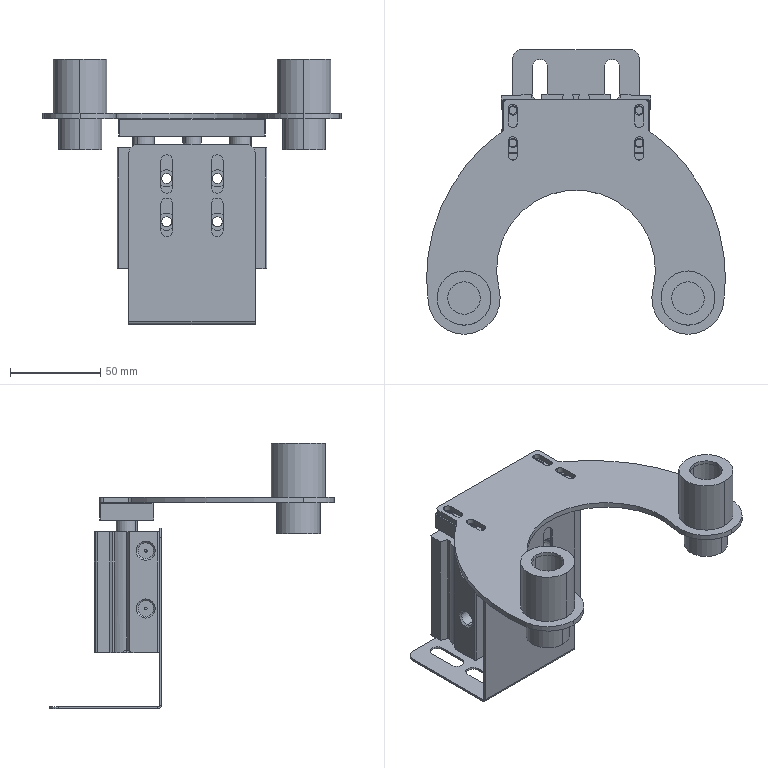Part | 17 solids | 668 faces | box 165.52 x 157.8 x 147 mm | volume 263535 mm3 | cylinder 302 | plane 248 | cone 103 | torus 12 | spline 3 | commonest cylinder face diameters 5 x57 4.2 x18 1.5 x16 3 x12 3.5 x12 8 x12